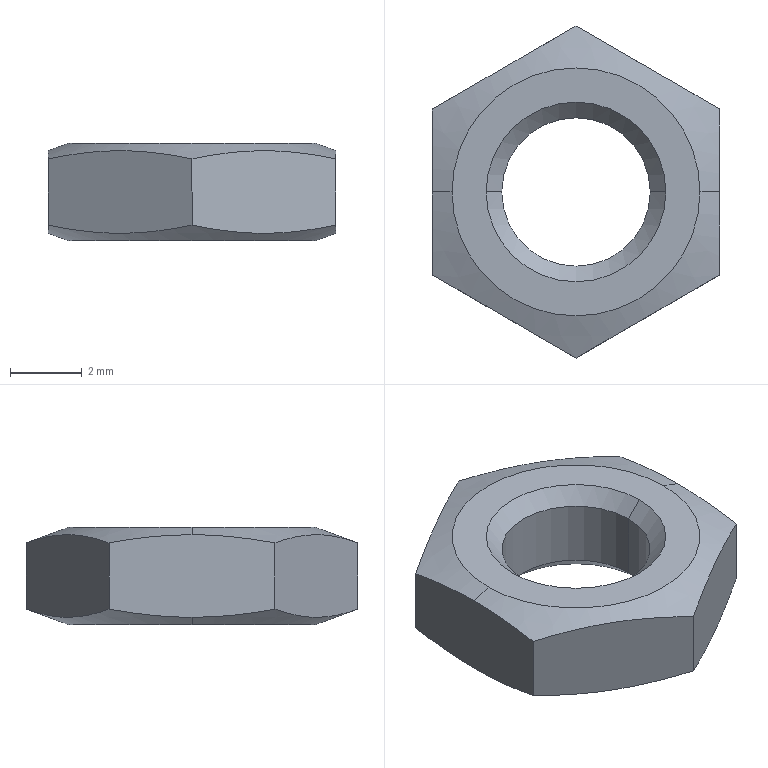Part | SolidWorks | features BaseBody 1 | 1 solid | 18 faces | box 8 x 9.238 x 2.7 mm | volume 105.377 mm3 | cone 8 | plane 8 | cylinder 2 | commonest cylinder face diameters 4.134 x2
STEP:
#1=CARTESIAN_POINT('',(-2.067,0.,0.433));
#2=VERTEX_POINT('',#1);
#3=CARTESIAN_POINT('',(2.067,0.,0.433));
#4=VERTEX_POINT('',#3);
#5=CARTESIAN_POINT('',(0.,0.,0.433));
#6=DIRECTION('',(0.,0.,1.));
#7=DIRECTION('',(1.,0.,0.));
#8=AXIS2_PLACEMENT_3D('',#5,#6,#7);
#9=CIRCLE('',#8,2.067);
#10=EDGE_CURVE('',#2,#4,#9,.T.);
#11=ORIENTED_EDGE('',*,*,#10,.F.);
#12=CARTESIAN_POINT('',(-2.067,0.,2.267));
#13=VERTEX_POINT('',#12);
#14=CARTESIAN_POINT('',(-2.067,0.,0.));
#15=DIRECTION('',(0.,0.,1.));
#16=VECTOR('',#15,1000.);
#17=LINE('',#14,#16);
#18=EDGE_CURVE('',#2,#13,#17,.T.);
#19=ORIENTED_EDGE('',*,*,#18,.T.);
#20=CARTESIAN_POINT('',(2.067,0.,2.267));
#21=VERTEX_POINT('',#20);
#22=CARTESIAN_POINT('',(0.,0.,2.267));
#23=DIRECTION('',(0.,0.,-1.));
#24=DIRECTION('',(1.,0.,0.));
#25=AXIS2_PLACEMENT_3D('',#22,#23,#24);
#26=CIRCLE('',#25,2.067);
#27=EDGE_CURVE('',#21,#13,#26,.T.);
#28=ORIENTED_EDGE('',*,*,#27,.F.);
#29=CARTESIAN_POINT('',(2.067,0.,0.));
#30=DIRECTION('',(0.,0.,1.));
#31=VECTOR('',#30,1000.);
#32=LINE('',#29,#31);
#33=EDGE_CURVE('',#4,#21,#32,.T.);
#34=ORIENTED_EDGE('',*,*,#33,.F.);
#35=EDGE_LOOP('',(#11,#19,#28,#34));
#36=FACE_OUTER_BOUND('',#35,.T.);
#37=CARTESIAN_POINT('',(0.,0.,0.));
#38=DIRECTION('',(0.,0.,1.));
#39=DIRECTION('',(1.,0.,0.));
#40=AXIS2_PLACEMENT_3D('',#37,#38,#39);
#41=CYLINDRICAL_SURFACE('',#40,2.067);
#42=ADVANCED_FACE('',(#36),#41,.F.);
#43=ORIENTED_EDGE('',*,*,#27,.T.);
#44=CARTESIAN_POINT('',(-2.5,0.,2.7));
#45=VERTEX_POINT('',#44);
#46=CARTESIAN_POINT('',(-2.5,0.,2.7));
#47=DIRECTION('',(-0.7071,0.,0.7071));
#48=VECTOR('',#47,1000.);
#49=LINE('',#46,#48);
#50=EDGE_CURVE('',#13,#45,#49,.T.);
#51=ORIENTED_EDGE('',*,*,#50,.T.);
#52=CARTESIAN_POINT('',(2.5,0.,2.7));
#53=VERTEX_POINT('',#52);
#54=CARTESIAN_POINT('',(0.,0.,2.7));
#55=DIRECTION('',(0.,0.,-1.));
#56=DIRECTION('',(1.,0.,0.));
#57=AXIS2_PLACEMENT_3D('',#54,#55,#56);
#58=CIRCLE('',#57,2.5);
#59=EDGE_CURVE('',#53,#45,#58,.T.);
#60=ORIENTED_EDGE('',*,*,#59,.F.);
#61=CARTESIAN_POINT('',(2.5,0.,2.7));
#62=DIRECTION('',(0.7071,0.,0.7071));
#63=VECTOR('',#62,1000.);
#64=LINE('',#61,#63);
#65=EDGE_CURVE('',#21,#53,#64,.T.);
#66=ORIENTED_EDGE('',*,*,#65,.F.);
#67=EDGE_LOOP('',(#43,#51,#60,#66));
#68=FACE_OUTER_BOUND('',#67,.T.);
#69=CARTESIAN_POINT('',(0.,0.,2.7));
#70=DIRECTION('',(0.,0.,1.));
#71=DIRECTION('',(1.,0.,0.));
#72=AXIS2_PLACEMENT_3D('',#69,#70,#71);
#73=CONICAL_SURFACE('',#72,2.5,0.7854);
#74=ADVANCED_FACE('',(#68),#73,.F.);
#75=ORIENTED_EDGE('',*,*,#10,.T.);
#76=CARTESIAN_POINT('',(2.5,0.,0.));
#77=VERTEX_POINT('',#76);
#78=CARTESIAN_POINT('',(2.5,0.,0.));
#79=DIRECTION('',(0.7071,0.,-0.7071));
#80=VECTOR('',#79,1000.);
#81=LINE('',#78,#80);
#82=EDGE_CURVE('',#4,#77,#81,.T.);
#83=ORIENTED_EDGE('',*,*,#82,.T.);
#84=CARTESIAN_POINT('',(-2.5,0.,0.));
#85=VERTEX_POINT('',#84);
#86=CARTESIAN_POINT('',(0.,0.,0.));
#87=DIRECTION('',(0.,0.,1.));
#88=DIRECTION('',(-1.,0.,0.));
#89=AXIS2_PLACEMENT_3D('',#86,#87,#88);
#90=CIRCLE('',#89,2.5);
#91=EDGE_CURVE('',#85,#77,#90,.T.);
#92=ORIENTED_EDGE('',*,*,#91,.F.);
#93=CARTESIAN_POINT('',(-2.5,0.,0.));
#94=DIRECTION('',(-0.7071,0.,-0.7071));
#95=VECTOR('',#94,1000.);
#96=LINE('',#93,#95);
#97=EDGE_CURVE('',#2,#85,#96,.T.);
#98=ORIENTED_EDGE('',*,*,#97,.F.);
#99=EDGE_LOOP('',(#75,#83,#92,#98));
#100=FACE_OUTER_BOUND('',#99,.T.);
#101=CARTESIAN_POINT('',(0.,0.,0.));
#102=DIRECTION('',(0.,0.,-1.));
#103=DIRECTION('',(-1.,0.,0.));
#104=AXIS2_PLACEMENT_3D('',#101,#102,#103);
#105=CONICAL_SURFACE('',#104,2.5,0.7854);
#106=ADVANCED_FACE('',(#100),#105,.F.);
#107=CARTESIAN_POINT('',(3.45,0.,2.7));
#108=VERTEX_POINT('',#107);
#109=CARTESIAN_POINT('',(-3.45,0.,2.7));
#110=VERTEX_POINT('',#109);
#111=CARTESIAN_POINT('',(0.,0.,2.7));
#112=DIRECTION('',(0.,0.,1.));
#113=DIRECTION('',(-1.,0.,0.));
#114=AXIS2_PLACEMENT_3D('',#111,#112,#113);
#115=CIRCLE('',#114,3.45);
#116=EDGE_CURVE('',#108,#110,#115,.T.);
#117=ORIENTED_EDGE('',*,*,#116,.F.);
#118=CARTESIAN_POINT('',(4.,0.,2.5));
#119=VERTEX_POINT('',#118);
#120=CARTESIAN_POINT('',(4.626,0.,2.272));
#121=DIRECTION('',(0.9397,0.,-0.342));
#122=VECTOR('',#121,1000.);
#123=LINE('',#120,#122);
#124=EDGE_CURVE('',#108,#119,#123,.T.);
#125=ORIENTED_EDGE('',*,*,#124,.T.);
#126=CARTESIAN_POINT('',(4.,2.309,2.275));
#127=VERTEX_POINT('',#126);
#128=CARTESIAN_POINT('',(4.,0.,2.5));
#129=CARTESIAN_POINT('',(4.,0.7698,2.5));
#130=CARTESIAN_POINT('',(4.,1.54,2.415));
#131=CARTESIAN_POINT('',(4.,2.309,2.275));
#132=B_SPLINE_CURVE_WITH_KNOTS('',3,(#128,#129,#130,#131),.UNSPECIFIED.,.F.,.F.,(4,4),(0.002309,0.004619),.UNSPECIFIED.);
#133=EDGE_CURVE('',#119,#127,#132,.T.);
#134=ORIENTED_EDGE('',*,*,#133,.T.);
#135=CARTESIAN_POINT('',(0.000000041,4.619,2.275));
#136=VERTEX_POINT('',#135);
#137=CARTESIAN_POINT('',(4.,2.309,2.275));
#138=CARTESIAN_POINT('',(3.333,2.694,2.415));
#139=CARTESIAN_POINT('',(2.,3.464,2.585));
#140=CARTESIAN_POINT('',(0.6667,4.234,2.415));
#141=CARTESIAN_POINT('',(0.000000041,4.619,2.275));
#142=B_SPLINE_CURVE_WITH_KNOTS('',3,(#137,#138,#139,#140,#141),.UNSPECIFIED.,.F.,.F.,(4,1,4),(0.,0.002309,0.004619),.UNSPECIFIED.);
#143=EDGE_CURVE('',#127,#136,#142,.T.);
#144=ORIENTED_EDGE('',*,*,#143,.T.);
#145=CARTESIAN_POINT('',(-4.,2.309,2.275));
#146=VERTEX_POINT('',#145);
#147=CARTESIAN_POINT('',(0.000000041,4.619,2.275));
#148=CARTESIAN_POINT('',(-0.6667,4.234,2.415));
#149=CARTESIAN_POINT('',(-2.,3.464,2.585));
#150=CARTESIAN_POINT('',(-3.333,2.694,2.415));
#151=CARTESIAN_POINT('',(-4.,2.309,2.275));
#152=B_SPLINE_CURVE_WITH_KNOTS('',3,(#147,#148,#149,#150,#151),.UNSPECIFIED.,.F.,.F.,(4,1,4),(0.,0.002309,0.004619),.UNSPECIFIED.);
#153=EDGE_CURVE('',#136,#146,#152,.T.);
#154=ORIENTED_EDGE('',*,*,#153,.T.);
#155=CARTESIAN_POINT('',(-4.,0.,2.5));
#156=VERTEX_POINT('',#155);
#157=CARTESIAN_POINT('',(-4.,2.309,2.275));
#158=CARTESIAN_POINT('',(-4.,1.54,2.415));
#159=CARTESIAN_POINT('',(-4.,0.7698,2.5));
#160=CARTESIAN_POINT('',(-4.,0.,2.5));
#161=B_SPLINE_CURVE_WITH_KNOTS('',3,(#157,#158,#159,#160),.UNSPECIFIED.,.F.,.F.,(4,4),(0.,0.002309),.UNSPECIFIED.);
#162=EDGE_CURVE('',#146,#156,#161,.T.);
#163=ORIENTED_EDGE('',*,*,#162,.T.);
#164=CARTESIAN_POINT('',(-4.626,0.,2.272));
#165=DIRECTION('',(-0.9397,0.,-0.342));
#166=VECTOR('',#165,1000.);
#167=LINE('',#164,#166);
#168=EDGE_CURVE('',#110,#156,#167,.T.);
#169=ORIENTED_EDGE('',*,*,#168,.F.);
#170=EDGE_LOOP('',(#117,#125,#134,#144,#154,#163,#169));
#171=FACE_OUTER_BOUND('',#170,.T.);
#172=CARTESIAN_POINT('',(0.,0.,2.272));
#173=DIRECTION('',(0.,0.,-1.));
#174=DIRECTION('',(-1.,0.,0.));
#175=AXIS2_PLACEMENT_3D('',#172,#173,#174);
#176=CONICAL_SURFACE('',#175,4.626,1.222);
#177=ADVANCED_FACE('',(#171),#176,.T.);
#178=CARTESIAN_POINT('',(3.45,0.,0.));
#179=VERTEX_POINT('',#178);
#180=CARTESIAN_POINT('',(-3.45,0.,0.));
#181=VERTEX_POINT('',#180);
#182=CARTESIAN_POINT('',(0.,0.,0.));
#183=DIRECTION('',(0.,0.,1.));
#184=DIRECTION('',(1.,0.,0.));
#185=AXIS2_PLACEMENT_3D('',#182,#183,#184);
#186=CIRCLE('',#185,3.45);
#187=EDGE_CURVE('',#179,#181,#186,.T.);
#188=ORIENTED_EDGE('',*,*,#187,.T.);
#189=CARTESIAN_POINT('',(-4.,0.,0.2002));
#190=VERTEX_POINT('',#189);
#191=CARTESIAN_POINT('',(-4.626,0.,0.428));
#192=DIRECTION('',(-0.9397,0.,0.342));
#193=VECTOR('',#192,1000.);
#194=LINE('',#191,#193);
#195=EDGE_CURVE('',#181,#190,#194,.T.);
#196=ORIENTED_EDGE('',*,*,#195,.T.);
#197=CARTESIAN_POINT('',(-4.,2.309,0.4254));
#198=VERTEX_POINT('',#197);
#199=CARTESIAN_POINT('',(-4.,0.,0.2002));
#200=CARTESIAN_POINT('',(-4.,0.7698,0.2002));
#201=CARTESIAN_POINT('',(-4.,1.54,0.2853));
#202=CARTESIAN_POINT('',(-4.,2.309,0.4254));
#203=B_SPLINE_CURVE_WITH_KNOTS('',3,(#199,#200,#201,#202),.UNSPECIFIED.,.F.,.F.,(4,4),(0.002309,0.004619),.UNSPECIFIED.);
#204=EDGE_CURVE('',#190,#198,#203,.T.);
#205=ORIENTED_EDGE('',*,*,#204,.T.);
#206=CARTESIAN_POINT('',(-0.000000041,4.619,0.4254));
#207=VERTEX_POINT('',#206);
#208=CARTESIAN_POINT('',(-4.,2.309,0.4254));
#209=CARTESIAN_POINT('',(-3.333,2.694,0.2853));
#210=CARTESIAN_POINT('',(-2.,3.464,0.1151));
#211=CARTESIAN_POINT('',(-0.6667,4.234,0.2853));
#212=CARTESIAN_POINT('',(-0.000000041,4.619,0.4254));
#213=B_SPLINE_CURVE_WITH_KNOTS('',3,(#208,#209,#210,#211,#212),.UNSPECIFIED.,.F.,.F.,(4,1,4),(0.,0.002309,0.004619),.UNSPECIFIED.);
#214=EDGE_CURVE('',#198,#207,#213,.T.);
#215=ORIENTED_EDGE('',*,*,#214,.T.);
#216=CARTESIAN_POINT('',(4.,2.309,0.4254));
#217=VERTEX_POINT('',#216);
#218=CARTESIAN_POINT('',(-0.000000041,4.619,0.4254));
#219=CARTESIAN_POINT('',(0.6667,4.234,0.2853));
#220=CARTESIAN_POINT('',(2.,3.464,0.1151));
#221=CARTESIAN_POINT('',(3.333,2.694,0.2853));
#222=CARTESIAN_POINT('',(4.,2.309,0.4254));
#223=B_SPLINE_CURVE_WITH_KNOTS('',3,(#218,#219,#220,#221,#222),.UNSPECIFIED.,.F.,.F.,(4,1,4),(0.,0.002309,0.004619),.UNSPECIFIED.);
#224=EDGE_CURVE('',#207,#217,#223,.T.);
#225=ORIENTED_EDGE('',*,*,#224,.T.);
#226=CARTESIAN_POINT('',(4.,0.,0.2002));
#227=VERTEX_POINT('',#226);
#228=CARTESIAN_POINT('',(4.,2.309,0.4254));
#229=CARTESIAN_POINT('',(4.,1.54,0.2853));
#230=CARTESIAN_POINT('',(4.,0.7698,0.2002));
#231=CARTESIAN_POINT('',(4.,0.,0.2002));
#232=B_SPLINE_CURVE_WITH_KNOTS('',3,(#228,#229,#230,#231),.UNSPECIFIED.,.F.,.F.,(4,4),(0.,0.002309),.UNSPECIFIED.);
#233=EDGE_CURVE('',#217,#227,#232,.T.);
#234=ORIENTED_EDGE('',*,*,#233,.T.);
#235=CARTESIAN_POINT('',(4.626,0.,0.428));
#236=DIRECTION('',(0.9397,0.,0.342));
#237=VECTOR('',#236,1000.);
#238=LINE('',#235,#237);
#239=EDGE_CURVE('',#179,#227,#238,.T.);
#240=ORIENTED_EDGE('',*,*,#239,.F.);
#241=EDGE_LOOP('',(#188,#196,#205,#215,#225,#234,#240));
#242=FACE_OUTER_BOUND('',#241,.T.);
#243=CARTESIAN_POINT('',(0.,0.,0.428));
#244=DIRECTION('',(0.,0.,1.));
#245=DIRECTION('',(1.,0.,0.));
#246=AXIS2_PLACEMENT_3D('',#243,#244,#245);
#247=CONICAL_SURFACE('',#246,4.626,1.222);
#248=ADVANCED_FACE('',(#242),#247,.T.);
#249=ORIENTED_EDGE('',*,*,#18,.F.);
#250=CARTESIAN_POINT('',(0.,0.,0.433));
#251=DIRECTION('',(0.,0.,1.));
#252=DIRECTION('',(1.,0.,0.));
#253=AXIS2_PLACEMENT_3D('',#250,#251,#252);
#254=CIRCLE('',#253,2.067);
#255=EDGE_CURVE('',#4,#2,#254,.T.);
#256=ORIENTED_EDGE('',*,*,#255,.F.);
#257=ORIENTED_EDGE('',*,*,#33,.T.);
#258=CARTESIAN_POINT('',(0.,0.,2.267));
#259=DIRECTION('',(0.,0.,-1.));
#260=DIRECTION('',(1.,0.,0.));
#261=AXIS2_PLACEMENT_3D('',#258,#259,#260);
#262=CIRCLE('',#261,2.067);
#263=EDGE_CURVE('',#13,#21,#262,.T.);
#264=ORIENTED_EDGE('',*,*,#263,.F.);
#265=EDGE_LOOP('',(#249,#256,#257,#264));
#266=FACE_OUTER_BOUND('',#265,.T.);
#267=CARTESIAN_POINT('',(0.,0.,0.));
#268=DIRECTION('',(0.,0.,1.));
#269=DIRECTION('',(1.,0.,0.));
#270=AXIS2_PLACEMENT_3D('',#267,#268,#269);
#271=CYLINDRICAL_SURFACE('',#270,2.067);
#272=ADVANCED_FACE('',(#266),#271,.F.);
#273=ORIENTED_EDGE('',*,*,#50,.F.);
#274=ORIENTED_EDGE('',*,*,#263,.T.);
#275=ORIENTED_EDGE('',*,*,#65,.T.);
#276=CARTESIAN_POINT('',(0.,0.,2.7));
#277=DIRECTION('',(0.,0.,-1.));
#278=DIRECTION('',(1.,0.,0.));
#279=AXIS2_PLACEMENT_3D('',#276,#277,#278);
#280=CIRCLE('',#279,2.5);
#281=EDGE_CURVE('',#45,#53,#280,.T.);
#282=ORIENTED_EDGE('',*,*,#281,.F.);
#283=EDGE_LOOP('',(#273,#274,#275,#282));
#284=FACE_OUTER_BOUND('',#283,.T.);
#285=CARTESIAN_POINT('',(0.,0.,2.7));
#286=DIRECTION('',(0.,0.,1.));
#287=DIRECTION('',(1.,0.,0.));
#288=AXIS2_PLACEMENT_3D('',#285,#286,#287);
#289=CONICAL_SURFACE('',#288,2.5,0.7854);
#290=ADVANCED_FACE('',(#284),#289,.F.);
#291=ORIENTED_EDGE('',*,*,#82,.F.);
#292=ORIENTED_EDGE('',*,*,#255,.T.);
#293=ORIENTED_EDGE('',*,*,#97,.T.);
#294=CARTESIAN_POINT('',(0.,0.,0.));
#295=DIRECTION('',(0.,0.,1.));
#296=DIRECTION('',(-1.,0.,0.));
#297=AXIS2_PLACEMENT_3D('',#294,#295,#296);
#298=CIRCLE('',#297,2.5);
#299=EDGE_CURVE('',#77,#85,#298,.T.);
#300=ORIENTED_EDGE('',*,*,#299,.F.);
#301=EDGE_LOOP('',(#291,#292,#293,#300));
#302=FACE_OUTER_BOUND('',#301,.T.);
#303=CARTESIAN_POINT('',(0.,0.,0.));
#304=DIRECTION('',(0.,0.,-1.));
#305=DIRECTION('',(-1.,0.,0.));
#306=AXIS2_PLACEMENT_3D('',#303,#304,#305);
#307=CONICAL_SURFACE('',#306,2.5,0.7854);
#308=ADVANCED_FACE('',(#302),#307,.F.);
#309=ORIENTED_EDGE('',*,*,#59,.T.);
#310=ORIENTED_EDGE('',*,*,#281,.T.);
#311=EDGE_LOOP('',(#309,#310));
#312=FACE_BOUND('',#311,.T.);
#313=CARTESIAN_POINT('',(0.,0.,2.7));
#314=DIRECTION('',(0.,0.,1.));
#315=DIRECTION('',(-1.,0.,0.));
#316=AXIS2_PLACEMENT_3D('',#313,#314,#315);
#317=CIRCLE('',#316,3.45);
#318=EDGE_CURVE('',#110,#108,#317,.T.);
#319=ORIENTED_EDGE('',*,*,#318,.T.);
#320=ORIENTED_EDGE('',*,*,#116,.T.);
#321=EDGE_LOOP('',(#319,#320));
#322=FACE_OUTER_BOUND('',#321,.T.);
#323=CARTESIAN_POINT('',(0.,0.,2.7));
#324=DIRECTION('',(0.,0.,1.));
#325=DIRECTION('',(1.,0.,0.));
#326=AXIS2_PLACEMENT_3D('',#323,#324,#325);
#327=PLANE('',#326);
#328=ADVANCED_FACE('',(#312,#322),#327,.T.);
#329=ORIENTED_EDGE('',*,*,#91,.T.);
#330=ORIENTED_EDGE('',*,*,#299,.T.);
#331=EDGE_LOOP('',(#329,#330));
#332=FACE_BOUND('',#331,.T.);
#333=ORIENTED_EDGE('',*,*,#187,.F.);
#334=CARTESIAN_POINT('',(0.,0.,0.));
#335=DIRECTION('',(0.,0.,1.));
#336=DIRECTION('',(1.,0.,0.));
#337=AXIS2_PLACEMENT_3D('',#334,#335,#336);
#338=CIRCLE('',#337,3.45);
#339=EDGE_CURVE('',#181,#179,#338,.T.);
#340=ORIENTED_EDGE('',*,*,#339,.F.);
#341=EDGE_LOOP('',(#333,#340));
#342=FACE_OUTER_BOUND('',#341,.T.);
#343=CARTESIAN_POINT('',(0.,0.,0.));
#344=DIRECTION('',(0.,0.,1.));
#345=DIRECTION('',(1.,0.,0.));
#346=AXIS2_PLACEMENT_3D('',#343,#344,#345);
#347=PLANE('',#346);
#348=ADVANCED_FACE('',(#332,#342),#347,.F.);
#349=ORIENTED_EDGE('',*,*,#124,.F.);
#350=ORIENTED_EDGE('',*,*,#318,.F.);
#351=ORIENTED_EDGE('',*,*,#168,.T.);
#352=CARTESIAN_POINT('',(-4.,-2.309,2.275));
#353=VERTEX_POINT('',#352);
#354=CARTESIAN_POINT('',(-4.,0.,2.5));
#355=CARTESIAN_POINT('',(-4.,-0.7698,2.5));
#356=CARTESIAN_POINT('',(-4.,-1.54,2.415));
#357=CARTESIAN_POINT('',(-4.,-2.309,2.275));
#358=B_SPLINE_CURVE_WITH_KNOTS('',3,(#354,#355,#356,#357),.UNSPECIFIED.,.F.,.F.,(4,4),(0.002309,0.004619),.UNSPECIFIED.);
#359=EDGE_CURVE('',#156,#353,#358,.T.);
#360=ORIENTED_EDGE('',*,*,#359,.T.);
#361=CARTESIAN_POINT('',(-0.000000041,-4.619,2.275));
#362=VERTEX_POINT('',#361);
#363=CARTESIAN_POINT('',(-4.,-2.309,2.275));
#364=CARTESIAN_POINT('',(-3.333,-2.694,2.415));
#365=CARTESIAN_POINT('',(-2.,-3.464,2.585));
#366=CARTESIAN_POINT('',(-0.6667,-4.234,2.415));
#367=CARTESIAN_POINT('',(-0.000000041,-4.619,2.275));
#368=B_SPLINE_CURVE_WITH_KNOTS('',3,(#363,#364,#365,#366,#367),.UNSPECIFIED.,.F.,.F.,(4,1,4),(0.,0.002309,0.004619),.UNSPECIFIED.);
#369=EDGE_CURVE('',#353,#362,#368,.T.);
#370=ORIENTED_EDGE('',*,*,#369,.T.);
#371=CARTESIAN_POINT('',(4.,-2.309,2.275));
#372=VERTEX_POINT('',#371);
#373=CARTESIAN_POINT('',(-0.000000041,-4.619,2.275));
#374=CARTESIAN_POINT('',(0.6667,-4.234,2.415));
#375=CARTESIAN_POINT('',(2.,-3.464,2.585));
#376=CARTESIAN_POINT('',(3.333,-2.694,2.415));
#377=CARTESIAN_POINT('',(4.,-2.309,2.275));
#378=B_SPLINE_CURVE_WITH_KNOTS('',3,(#373,#374,#375,#376,#377),.UNSPECIFIED.,.F.,.F.,(4,1,4),(0.,0.002309,0.004619),.UNSPECIFIED.);
#379=EDGE_CURVE('',#362,#372,#378,.T.);
#380=ORIENTED_EDGE('',*,*,#379,.T.);
#381=CARTESIAN_POINT('',(4.,-2.309,2.275));
#382=CARTESIAN_POINT('',(4.,-1.54,2.415));
#383=CARTESIAN_POINT('',(4.,-0.7698,2.5));
#384=CARTESIAN_POINT('',(4.,0.,2.5));
#385=B_SPLINE_CURVE_WITH_KNOTS('',3,(#381,#382,#383,#384),.UNSPECIFIED.,.F.,.F.,(4,4),(0.,0.002309),.UNSPECIFIED.);
#386=EDGE_CURVE('',#372,#119,#385,.T.);
#387=ORIENTED_EDGE('',*,*,#386,.T.);
#388=EDGE_LOOP('',(#349,#350,#351,#360,#370,#380,#387));
#389=FACE_OUTER_BOUND('',#388,.T.);
#390=CARTESIAN_POINT('',(0.,0.,2.272));
#391=DIRECTION('',(0.,0.,-1.));
#392=DIRECTION('',(-1.,0.,0.));
#393=AXIS2_PLACEMENT_3D('',#390,#391,#392);
#394=CONICAL_SURFACE('',#393,4.626,1.222);
#395=ADVANCED_FACE('',(#389),#394,.T.);
#396=ORIENTED_EDGE('',*,*,#195,.F.);
#397=ORIENTED_EDGE('',*,*,#339,.T.);
#398=ORIENTED_EDGE('',*,*,#239,.T.);
#399=CARTESIAN_POINT('',(4.,-2.309,0.4254));
#400=VERTEX_POINT('',#399);
#401=CARTESIAN_POINT('',(4.,0.,0.2002));
#402=CARTESIAN_POINT('',(4.,-0.7698,0.2002));
#403=CARTESIAN_POINT('',(4.,-1.54,0.2853));
#404=CARTESIAN_POINT('',(4.,-2.309,0.4254));
#405=B_SPLINE_CURVE_WITH_KNOTS('',3,(#401,#402,#403,#404),.UNSPECIFIED.,.F.,.F.,(4,4),(0.002309,0.004619),.UNSPECIFIED.);
#406=EDGE_CURVE('',#227,#400,#405,.T.);
#407=ORIENTED_EDGE('',*,*,#406,.T.);
#408=CARTESIAN_POINT('',(0.000000041,-4.619,0.4254));
#409=VERTEX_POINT('',#408);
#410=CARTESIAN_POINT('',(4.,-2.309,0.4254));
#411=CARTESIAN_POINT('',(3.333,-2.694,0.2853));
#412=CARTESIAN_POINT('',(2.,-3.464,0.1151));
#413=CARTESIAN_POINT('',(0.6667,-4.234,0.2853));
#414=CARTESIAN_POINT('',(0.000000041,-4.619,0.4254));
#415=B_SPLINE_CURVE_WITH_KNOTS('',3,(#410,#411,#412,#413,#414),.UNSPECIFIED.,.F.,.F.,(4,1,4),(0.,0.002309,0.004619),.UNSPECIFIED.);
#416=EDGE_CURVE('',#400,#409,#415,.T.);
#417=ORIENTED_EDGE('',*,*,#416,.T.);
#418=CARTESIAN_POINT('',(-4.,-2.309,0.4254));
#419=VERTEX_POINT('',#418);
#420=CARTESIAN_POINT('',(0.000000041,-4.619,0.4254));
#421=CARTESIAN_POINT('',(-0.6667,-4.234,0.2853));
#422=CARTESIAN_POINT('',(-2.,-3.464,0.1151));
#423=CARTESIAN_POINT('',(-3.333,-2.694,0.2853));
#424=CARTESIAN_POINT('',(-4.,-2.309,0.4254));
#425=B_SPLINE_CURVE_WITH_KNOTS('',3,(#420,#421,#422,#423,#424),.UNSPECIFIED.,.F.,.F.,(4,1,4),(0.,0.002309,0.004619),.UNSPECIFIED.);
#426=EDGE_CURVE('',#409,#419,#425,.T.);
#427=ORIENTED_EDGE('',*,*,#426,.T.);
#428=CARTESIAN_POINT('',(-4.,-2.309,0.4254));
#429=CARTESIAN_POINT('',(-4.,-1.54,0.2853));
#430=CARTESIAN_POINT('',(-4.,-0.7698,0.2002));
#431=CARTESIAN_POINT('',(-4.,0.,0.2002));
#432=B_SPLINE_CURVE_WITH_KNOTS('',3,(#428,#429,#430,#431),.UNSPECIFIED.,.F.,.F.,(4,4),(0.,0.002309),.UNSPECIFIED.);
#433=EDGE_CURVE('',#419,#190,#432,.T.);
#434=ORIENTED_EDGE('',*,*,#433,.T.);
#435=EDGE_LOOP('',(#396,#397,#398,#407,#417,#427,#434));
#436=FACE_OUTER_BOUND('',#435,.T.);
#437=CARTESIAN_POINT('',(0.,0.,0.428));
#438=DIRECTION('',(0.,0.,1.));
#439=DIRECTION('',(1.,0.,0.));
#440=AXIS2_PLACEMENT_3D('',#437,#438,#439);
#441=CONICAL_SURFACE('',#440,4.626,1.222);
#442=ADVANCED_FACE('',(#436),#441,.T.);
#443=ORIENTED_EDGE('',*,*,#386,.F.);
#444=CARTESIAN_POINT('',(4.,-2.309,2.7));
#445=DIRECTION('',(0.,0.,1.));
#446=VECTOR('',#445,1000.);
#447=LINE('',#444,#446);
#448=EDGE_CURVE('',#400,#372,#447,.T.);
#449=ORIENTED_EDGE('',*,*,#448,.F.);
#450=ORIENTED_EDGE('',*,*,#406,.F.);
#451=ORIENTED_EDGE('',*,*,#233,.F.);
#452=CARTESIAN_POINT('',(4.,2.309,2.7));
#453=DIRECTION('',(0.,0.,-1.));
#454=VECTOR('',#453,1000.);
#455=LINE('',#452,#454);
#456=EDGE_CURVE('',#127,#217,#455,.T.);
#457=ORIENTED_EDGE('',*,*,#456,.F.);
#458=ORIENTED_EDGE('',*,*,#133,.F.);
#459=EDGE_LOOP('',(#443,#449,#450,#451,#457,#458));
#460=FACE_OUTER_BOUND('',#459,.T.);
#461=CARTESIAN_POINT('',(4.,-2.309,2.7));
#462=DIRECTION('',(-1.,0.,0.));
#463=DIRECTION('',(0.,0.,1.));
#464=AXIS2_PLACEMENT_3D('',#461,#462,#463);
#465=PLANE('',#464);
#466=ADVANCED_FACE('',(#460),#465,.F.);
#467=ORIENTED_EDGE('',*,*,#379,.F.);
#468=CARTESIAN_POINT('',(0.,-4.619,2.7));
#469=DIRECTION('',(0.,0.,1.));
#470=VECTOR('',#469,1000.);
#471=LINE('',#468,#470);
#472=EDGE_CURVE('',#409,#362,#471,.T.);
#473=ORIENTED_EDGE('',*,*,#472,.F.);
#474=ORIENTED_EDGE('',*,*,#416,.F.);
#475=ORIENTED_EDGE('',*,*,#448,.T.);
#476=EDGE_LOOP('',(#467,#473,#474,#475));
#477=FACE_OUTER_BOUND('',#476,.T.);
#478=CARTESIAN_POINT('',(0.,-4.619,2.7));
#479=DIRECTION('',(-0.5,0.866,0.));
#480=DIRECTION('',(-0.866,-0.5,0.));
#481=AXIS2_PLACEMENT_3D('',#478,#479,#480);
#482=PLANE('',#481);
#483=ADVANCED_FACE('',(#477),#482,.F.);
#484=ORIENTED_EDGE('',*,*,#369,.F.);
#485=CARTESIAN_POINT('',(-4.,-2.309,2.7));
#486=DIRECTION('',(0.,0.,1.));
#487=VECTOR('',#486,1000.);
#488=LINE('',#485,#487);
#489=EDGE_CURVE('',#419,#353,#488,.T.);
#490=ORIENTED_EDGE('',*,*,#489,.F.);
#491=ORIENTED_EDGE('',*,*,#426,.F.);
#492=ORIENTED_EDGE('',*,*,#472,.T.);
#493=EDGE_LOOP('',(#484,#490,#491,#492));
#494=FACE_OUTER_BOUND('',#493,.T.);
#495=CARTESIAN_POINT('',(-4.,-2.309,2.7));
#496=DIRECTION('',(0.5,0.866,0.));
#497=DIRECTION('',(-0.866,0.5,0.));
#498=AXIS2_PLACEMENT_3D('',#495,#496,#497);
#499=PLANE('',#498);
#500=ADVANCED_FACE('',(#494),#499,.F.);
#501=ORIENTED_EDGE('',*,*,#162,.F.);
#502=CARTESIAN_POINT('',(-4.,2.309,2.7));
#503=DIRECTION('',(0.,0.,1.));
#504=VECTOR('',#503,1000.);
#505=LINE('',#502,#504);
#506=EDGE_CURVE('',#198,#146,#505,.T.);
#507=ORIENTED_EDGE('',*,*,#506,.F.);
#508=ORIENTED_EDGE('',*,*,#204,.F.);
#509=ORIENTED_EDGE('',*,*,#433,.F.);
#510=ORIENTED_EDGE('',*,*,#489,.T.);
#511=ORIENTED_EDGE('',*,*,#359,.F.);
#512=EDGE_LOOP('',(#501,#507,#508,#509,#510,#511));
#513=FACE_OUTER_BOUND('',#512,.T.);
#514=CARTESIAN_POINT('',(-4.,2.309,2.7));
#515=DIRECTION('',(1.,0.,0.));
#516=DIRECTION('',(0.,0.,-1.));
#517=AXIS2_PLACEMENT_3D('',#514,#515,#516);
#518=PLANE('',#517);
#519=ADVANCED_FACE('',(#513),#518,.F.);
#520=ORIENTED_EDGE('',*,*,#153,.F.);
#521=CARTESIAN_POINT('',(0.,4.619,2.7));
#522=DIRECTION('',(0.,0.,1.));
#523=VECTOR('',#522,1000.);
#524=LINE('',#521,#523);
#525=EDGE_CURVE('',#207,#136,#524,.T.);
#526=ORIENTED_EDGE('',*,*,#525,.F.);
#527=ORIENTED_EDGE('',*,*,#214,.F.);
#528=ORIENTED_EDGE('',*,*,#506,.T.);
#529=EDGE_LOOP('',(#520,#526,#527,#528));
#530=FACE_OUTER_BOUND('',#529,.T.);
#531=CARTESIAN_POINT('',(0.,4.619,2.7));
#532=DIRECTION('',(0.5,-0.866,0.));
#533=DIRECTION('',(0.866,0.5,0.));
#534=AXIS2_PLACEMENT_3D('',#531,#532,#533);
#535=PLANE('',#534);
#536=ADVANCED_FACE('',(#530),#535,.F.);
#537=ORIENTED_EDGE('',*,*,#143,.F.);
#538=ORIENTED_EDGE('',*,*,#456,.T.);
#539=ORIENTED_EDGE('',*,*,#224,.F.);
#540=ORIENTED_EDGE('',*,*,#525,.T.);
#541=EDGE_LOOP('',(#537,#538,#539,#540));
#542=FACE_OUTER_BOUND('',#541,.T.);
#543=CARTESIAN_POINT('',(4.,2.309,2.7));
#544=DIRECTION('',(-0.5,-0.866,0.));
#545=DIRECTION('',(0.866,-0.5,0.));
#546=AXIS2_PLACEMENT_3D('',#543,#544,#545);
#547=PLANE('',#546);
#548=ADVANCED_FACE('',(#542),#547,.F.);
#549=CLOSED_SHELL('',(#42,#74,#106,#177,#248,#272,#290,#308,#328,#348,#395,#442,#466,#483,#500,#519,#536,#548));
#550=MANIFOLD_SOLID_BREP('',#549);
#551=CARTESIAN_POINT('',(0.,0.,0.));
#552=DIRECTION('',(0.,0.,1.));
#553=DIRECTION('',(1.,0.,0.));
#554=AXIS2_PLACEMENT_3D('',#551,#552,#553);
#555=(LENGTH_UNIT()NAMED_UNIT(*)SI_UNIT(.MILLI.,.METRE.));
#556=UNCERTAINTY_MEASURE_WITH_UNIT(LENGTH_MEASURE(0.00001),#555,'','');
#557=(NAMED_UNIT(*)PLANE_ANGLE_UNIT()SI_UNIT($,.RADIAN.));
#558=(NAMED_UNIT(*)SI_UNIT($,.STERADIAN.)SOLID_ANGLE_UNIT());
#559=(GEOMETRIC_REPRESENTATION_CONTEXT(3)GLOBAL_UNCERTAINTY_ASSIGNED_CONTEXT((#556))GLOBAL_UNIT_ASSIGNED_CONTEXT((#555,#557,#558))REPRESENTATION_CONTEXT('',''));
#560=ADVANCED_BREP_SHAPE_REPRESENTATION('',(#550,#554),#559);